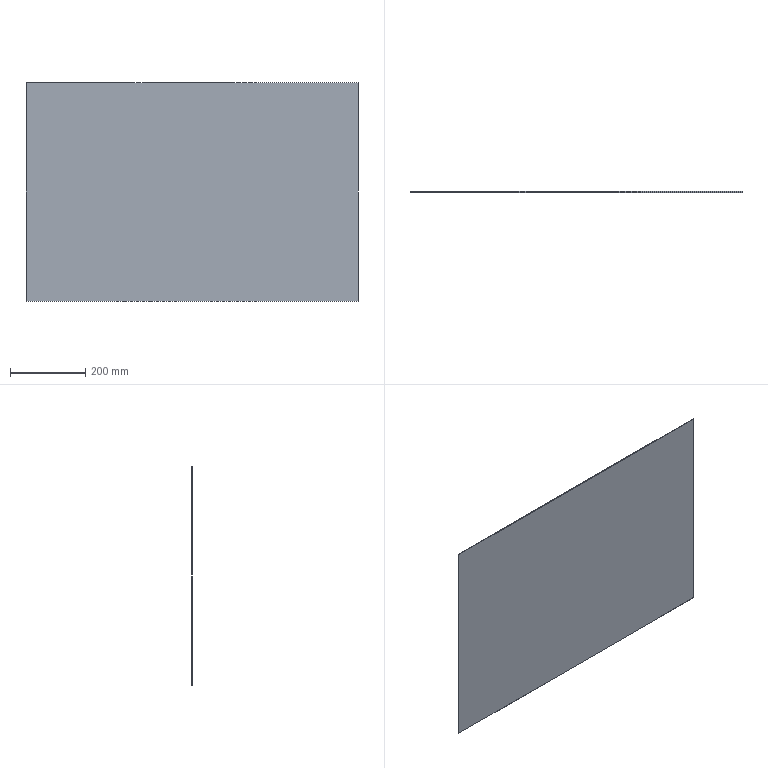Part | STEP file | 880X580 sealing plate | 1 solid | 6 faces | box 880 x 2 x 580 mm | volume 1020800 mm3 | plane 6
STEP:
#1=CARTESIAN_POINT('',(0.,0.,0.));
#2=DIRECTION('',(0.,0.,1.));
#3=DIRECTION('',(1.,0.,0.));
#4=AXIS2_PLACEMENT_3D('',#1,#2,#3);
#5=CARTESIAN_POINT('',(0.,0.,0.));
#6=VERTEX_POINT('',#5);
#7=CARTESIAN_POINT('',(0.,0.,580.));
#8=VERTEX_POINT('',#7);
#9=CARTESIAN_POINT('',(0.,0.,0.));
#10=DIRECTION('',(0.,0.,1.));
#11=VECTOR('',#10,1.);
#12=LINE('',#9,#11);
#13=CARTESIAN_POINT('',(0.,2.,0.));
#14=DIRECTION('',(1.,0.,0.));
#15=DIRECTION('',(0.,0.,-1.));
#16=AXIS2_PLACEMENT_3D('',#13,#14,#15);
#17=PLANE('',#16);
#18=CARTESIAN_POINT('',(0.,-2.));
#19=DIRECTION('',(-1.,0.));
#20=VECTOR('',#19,1.);
#21=LINE('',#18,#20);
#22=(GEOMETRIC_REPRESENTATION_CONTEXT(2)PARAMETRIC_REPRESENTATION_CONTEXT()REPRESENTATION_CONTEXT('',''));
#23=DEFINITIONAL_REPRESENTATION('',(#21),#22);
#24=PCURVE('',#17,#23);
#25=CARTESIAN_POINT('',(0.,0.,0.));
#26=DIRECTION('',(0.,1.,0.));
#27=DIRECTION('',(0.,0.,1.));
#28=AXIS2_PLACEMENT_3D('',#25,#26,#27);
#29=PLANE('',#28);
#30=CARTESIAN_POINT('',(0.,0.));
#31=DIRECTION('',(1.,0.));
#32=VECTOR('',#31,1.);
#33=LINE('',#30,#32);
#34=(GEOMETRIC_REPRESENTATION_CONTEXT(2)PARAMETRIC_REPRESENTATION_CONTEXT()REPRESENTATION_CONTEXT('',''));
#35=DEFINITIONAL_REPRESENTATION('',(#33),#34);
#36=PCURVE('',#29,#35);
#37=SURFACE_CURVE('',#12,(#24,#36),.PCURVE_S1.);
#38=EDGE_CURVE('',#6,#8,#37,.T.);
#39=ORIENTED_EDGE('',*,*,#38,.T.);
#40=CARTESIAN_POINT('',(0.,2.,580.));
#41=VERTEX_POINT('',#40);
#42=CARTESIAN_POINT('',(0.,2.,580.));
#43=DIRECTION('',(0.,-1.,0.));
#44=VECTOR('',#43,1.);
#45=LINE('',#42,#44);
#46=CARTESIAN_POINT('',(-580.,0.));
#47=DIRECTION('',(0.,-1.));
#48=VECTOR('',#47,1.);
#49=LINE('',#46,#48);
#50=(GEOMETRIC_REPRESENTATION_CONTEXT(2)PARAMETRIC_REPRESENTATION_CONTEXT()REPRESENTATION_CONTEXT('',''));
#51=DEFINITIONAL_REPRESENTATION('',(#49),#50);
#52=PCURVE('',#17,#51);
#53=CARTESIAN_POINT('',(0.,2.,580.));
#54=DIRECTION('',(0.,0.,-1.));
#55=DIRECTION('',(-1.,0.,0.));
#56=AXIS2_PLACEMENT_3D('',#53,#54,#55);
#57=PLANE('',#56);
#58=CARTESIAN_POINT('',(0.,0.));
#59=DIRECTION('',(0.,-1.));
#60=VECTOR('',#59,1.);
#61=LINE('',#58,#60);
#62=(GEOMETRIC_REPRESENTATION_CONTEXT(2)PARAMETRIC_REPRESENTATION_CONTEXT()REPRESENTATION_CONTEXT('',''));
#63=DEFINITIONAL_REPRESENTATION('',(#61),#62);
#64=PCURVE('',#57,#63);
#65=SURFACE_CURVE('',#45,(#52,#64),.PCURVE_S1.);
#66=EDGE_CURVE('',#41,#8,#65,.T.);
#67=ORIENTED_EDGE('',*,*,#66,.F.);
#68=CARTESIAN_POINT('',(0.,2.,0.));
#69=VERTEX_POINT('',#68);
#70=CARTESIAN_POINT('',(0.,2.,0.));
#71=DIRECTION('',(0.,0.,1.));
#72=VECTOR('',#71,1.);
#73=LINE('',#70,#72);
#74=CARTESIAN_POINT('',(0.,0.));
#75=DIRECTION('',(-1.,0.));
#76=VECTOR('',#75,1.);
#77=LINE('',#74,#76);
#78=(GEOMETRIC_REPRESENTATION_CONTEXT(2)PARAMETRIC_REPRESENTATION_CONTEXT()REPRESENTATION_CONTEXT('',''));
#79=DEFINITIONAL_REPRESENTATION('',(#77),#78);
#80=PCURVE('',#17,#79);
#81=CARTESIAN_POINT('',(0.,2.,0.));
#82=DIRECTION('',(0.,1.,0.));
#83=DIRECTION('',(0.,0.,1.));
#84=AXIS2_PLACEMENT_3D('',#81,#82,#83);
#85=PLANE('',#84);
#86=CARTESIAN_POINT('',(0.,0.));
#87=DIRECTION('',(1.,0.));
#88=VECTOR('',#87,1.);
#89=LINE('',#86,#88);
#90=(GEOMETRIC_REPRESENTATION_CONTEXT(2)PARAMETRIC_REPRESENTATION_CONTEXT()REPRESENTATION_CONTEXT('',''));
#91=DEFINITIONAL_REPRESENTATION('',(#89),#90);
#92=PCURVE('',#85,#91);
#93=SURFACE_CURVE('',#73,(#80,#92),.PCURVE_S1.);
#94=EDGE_CURVE('',#69,#41,#93,.T.);
#95=ORIENTED_EDGE('',*,*,#94,.F.);
#96=CARTESIAN_POINT('',(0.,2.,0.));
#97=DIRECTION('',(0.,-1.,0.));
#98=VECTOR('',#97,1.);
#99=LINE('',#96,#98);
#100=CARTESIAN_POINT('',(0.,0.));
#101=DIRECTION('',(0.,-1.));
#102=VECTOR('',#101,1.);
#103=LINE('',#100,#102);
#104=(GEOMETRIC_REPRESENTATION_CONTEXT(2)PARAMETRIC_REPRESENTATION_CONTEXT()REPRESENTATION_CONTEXT('',''));
#105=DEFINITIONAL_REPRESENTATION('',(#103),#104);
#106=PCURVE('',#17,#105);
#107=CARTESIAN_POINT('',(0.,2.,0.));
#108=DIRECTION('',(0.,0.,1.));
#109=DIRECTION('',(1.,0.,0.));
#110=AXIS2_PLACEMENT_3D('',#107,#108,#109);
#111=PLANE('',#110);
#112=CARTESIAN_POINT('',(0.,0.));
#113=DIRECTION('',(0.,-1.));
#114=VECTOR('',#113,1.);
#115=LINE('',#112,#114);
#116=(GEOMETRIC_REPRESENTATION_CONTEXT(2)PARAMETRIC_REPRESENTATION_CONTEXT()REPRESENTATION_CONTEXT('',''));
#117=DEFINITIONAL_REPRESENTATION('',(#115),#116);
#118=PCURVE('',#111,#117);
#119=SURFACE_CURVE('',#99,(#106,#118),.PCURVE_S1.);
#120=EDGE_CURVE('',#69,#6,#119,.T.);
#121=ORIENTED_EDGE('',*,*,#120,.T.);
#122=EDGE_LOOP('',(#39,#67,#95,#121));
#123=FACE_BOUND('',#122,.T.);
#124=ADVANCED_FACE('',(#123),#17,.F.);
#125=CARTESIAN_POINT('',(880.,0.,580.));
#126=VERTEX_POINT('',#125);
#127=CARTESIAN_POINT('',(0.,0.,580.));
#128=DIRECTION('',(1.,0.,0.));
#129=VECTOR('',#128,1.);
#130=LINE('',#127,#129);
#131=CARTESIAN_POINT('',(0.,-2.));
#132=DIRECTION('',(-1.,0.));
#133=VECTOR('',#132,1.);
#134=LINE('',#131,#133);
#135=(GEOMETRIC_REPRESENTATION_CONTEXT(2)PARAMETRIC_REPRESENTATION_CONTEXT()REPRESENTATION_CONTEXT('',''));
#136=DEFINITIONAL_REPRESENTATION('',(#134),#135);
#137=PCURVE('',#57,#136);
#138=CARTESIAN_POINT('',(580.,0.));
#139=DIRECTION('',(0.,1.));
#140=VECTOR('',#139,1.);
#141=LINE('',#138,#140);
#142=(GEOMETRIC_REPRESENTATION_CONTEXT(2)PARAMETRIC_REPRESENTATION_CONTEXT()REPRESENTATION_CONTEXT('',''));
#143=DEFINITIONAL_REPRESENTATION('',(#141),#142);
#144=PCURVE('',#29,#143);
#145=SURFACE_CURVE('',#130,(#137,#144),.PCURVE_S1.);
#146=EDGE_CURVE('',#8,#126,#145,.T.);
#147=ORIENTED_EDGE('',*,*,#146,.T.);
#148=CARTESIAN_POINT('',(880.,2.,580.));
#149=VERTEX_POINT('',#148);
#150=CARTESIAN_POINT('',(880.,2.,580.));
#151=DIRECTION('',(0.,-1.,0.));
#152=VECTOR('',#151,1.);
#153=LINE('',#150,#152);
#154=CARTESIAN_POINT('',(-880.,0.));
#155=DIRECTION('',(0.,-1.));
#156=VECTOR('',#155,1.);
#157=LINE('',#154,#156);
#158=(GEOMETRIC_REPRESENTATION_CONTEXT(2)PARAMETRIC_REPRESENTATION_CONTEXT()REPRESENTATION_CONTEXT('',''));
#159=DEFINITIONAL_REPRESENTATION('',(#157),#158);
#160=PCURVE('',#57,#159);
#161=CARTESIAN_POINT('',(880.,2.,0.));
#162=DIRECTION('',(-1.,0.,0.));
#163=DIRECTION('',(0.,0.,1.));
#164=AXIS2_PLACEMENT_3D('',#161,#162,#163);
#165=PLANE('',#164);
#166=CARTESIAN_POINT('',(580.,0.));
#167=DIRECTION('',(0.,-1.));
#168=VECTOR('',#167,1.);
#169=LINE('',#166,#168);
#170=(GEOMETRIC_REPRESENTATION_CONTEXT(2)PARAMETRIC_REPRESENTATION_CONTEXT()REPRESENTATION_CONTEXT('',''));
#171=DEFINITIONAL_REPRESENTATION('',(#169),#170);
#172=PCURVE('',#165,#171);
#173=SURFACE_CURVE('',#153,(#160,#172),.PCURVE_S1.);
#174=EDGE_CURVE('',#149,#126,#173,.T.);
#175=ORIENTED_EDGE('',*,*,#174,.F.);
#176=CARTESIAN_POINT('',(0.,2.,580.));
#177=DIRECTION('',(1.,0.,0.));
#178=VECTOR('',#177,1.);
#179=LINE('',#176,#178);
#180=CARTESIAN_POINT('',(0.,0.));
#181=DIRECTION('',(-1.,0.));
#182=VECTOR('',#181,1.);
#183=LINE('',#180,#182);
#184=(GEOMETRIC_REPRESENTATION_CONTEXT(2)PARAMETRIC_REPRESENTATION_CONTEXT()REPRESENTATION_CONTEXT('',''));
#185=DEFINITIONAL_REPRESENTATION('',(#183),#184);
#186=PCURVE('',#57,#185);
#187=CARTESIAN_POINT('',(580.,0.));
#188=DIRECTION('',(0.,1.));
#189=VECTOR('',#188,1.);
#190=LINE('',#187,#189);
#191=(GEOMETRIC_REPRESENTATION_CONTEXT(2)PARAMETRIC_REPRESENTATION_CONTEXT()REPRESENTATION_CONTEXT('',''));
#192=DEFINITIONAL_REPRESENTATION('',(#190),#191);
#193=PCURVE('',#85,#192);
#194=SURFACE_CURVE('',#179,(#186,#193),.PCURVE_S1.);
#195=EDGE_CURVE('',#41,#149,#194,.T.);
#196=ORIENTED_EDGE('',*,*,#195,.F.);
#197=ORIENTED_EDGE('',*,*,#66,.T.);
#198=EDGE_LOOP('',(#147,#175,#196,#197));
#199=FACE_BOUND('',#198,.T.);
#200=ADVANCED_FACE('',(#199),#57,.F.);
#201=CARTESIAN_POINT('',(880.,0.,0.));
#202=VERTEX_POINT('',#201);
#203=CARTESIAN_POINT('',(880.,0.,0.));
#204=DIRECTION('',(0.,0.,-1.));
#205=VECTOR('',#204,1.);
#206=LINE('',#203,#205);
#207=CARTESIAN_POINT('',(0.,-2.));
#208=DIRECTION('',(-1.,0.));
#209=VECTOR('',#208,1.);
#210=LINE('',#207,#209);
#211=(GEOMETRIC_REPRESENTATION_CONTEXT(2)PARAMETRIC_REPRESENTATION_CONTEXT()REPRESENTATION_CONTEXT('',''));
#212=DEFINITIONAL_REPRESENTATION('',(#210),#211);
#213=PCURVE('',#165,#212);
#214=CARTESIAN_POINT('',(0.,880.));
#215=DIRECTION('',(-1.,0.));
#216=VECTOR('',#215,1.);
#217=LINE('',#214,#216);
#218=(GEOMETRIC_REPRESENTATION_CONTEXT(2)PARAMETRIC_REPRESENTATION_CONTEXT()REPRESENTATION_CONTEXT('',''));
#219=DEFINITIONAL_REPRESENTATION('',(#217),#218);
#220=PCURVE('',#29,#219);
#221=SURFACE_CURVE('',#206,(#213,#220),.PCURVE_S1.);
#222=EDGE_CURVE('',#126,#202,#221,.T.);
#223=ORIENTED_EDGE('',*,*,#222,.T.);
#224=CARTESIAN_POINT('',(880.,2.,0.));
#225=VERTEX_POINT('',#224);
#226=CARTESIAN_POINT('',(880.,2.,0.));
#227=DIRECTION('',(0.,-1.,0.));
#228=VECTOR('',#227,1.);
#229=LINE('',#226,#228);
#230=CARTESIAN_POINT('',(0.,0.));
#231=DIRECTION('',(0.,-1.));
#232=VECTOR('',#231,1.);
#233=LINE('',#230,#232);
#234=(GEOMETRIC_REPRESENTATION_CONTEXT(2)PARAMETRIC_REPRESENTATION_CONTEXT()REPRESENTATION_CONTEXT('',''));
#235=DEFINITIONAL_REPRESENTATION('',(#233),#234);
#236=PCURVE('',#165,#235);
#237=CARTESIAN_POINT('',(880.,0.));
#238=DIRECTION('',(0.,-1.));
#239=VECTOR('',#238,1.);
#240=LINE('',#237,#239);
#241=(GEOMETRIC_REPRESENTATION_CONTEXT(2)PARAMETRIC_REPRESENTATION_CONTEXT()REPRESENTATION_CONTEXT('',''));
#242=DEFINITIONAL_REPRESENTATION('',(#240),#241);
#243=PCURVE('',#111,#242);
#244=SURFACE_CURVE('',#229,(#236,#243),.PCURVE_S1.);
#245=EDGE_CURVE('',#225,#202,#244,.T.);
#246=ORIENTED_EDGE('',*,*,#245,.F.);
#247=CARTESIAN_POINT('',(880.,2.,0.));
#248=DIRECTION('',(0.,0.,-1.));
#249=VECTOR('',#248,1.);
#250=LINE('',#247,#249);
#251=CARTESIAN_POINT('',(0.,0.));
#252=DIRECTION('',(-1.,0.));
#253=VECTOR('',#252,1.);
#254=LINE('',#251,#253);
#255=(GEOMETRIC_REPRESENTATION_CONTEXT(2)PARAMETRIC_REPRESENTATION_CONTEXT()REPRESENTATION_CONTEXT('',''));
#256=DEFINITIONAL_REPRESENTATION('',(#254),#255);
#257=PCURVE('',#165,#256);
#258=CARTESIAN_POINT('',(0.,880.));
#259=DIRECTION('',(-1.,0.));
#260=VECTOR('',#259,1.);
#261=LINE('',#258,#260);
#262=(GEOMETRIC_REPRESENTATION_CONTEXT(2)PARAMETRIC_REPRESENTATION_CONTEXT()REPRESENTATION_CONTEXT('',''));
#263=DEFINITIONAL_REPRESENTATION('',(#261),#262);
#264=PCURVE('',#85,#263);
#265=SURFACE_CURVE('',#250,(#257,#264),.PCURVE_S1.);
#266=EDGE_CURVE('',#149,#225,#265,.T.);
#267=ORIENTED_EDGE('',*,*,#266,.F.);
#268=ORIENTED_EDGE('',*,*,#174,.T.);
#269=EDGE_LOOP('',(#223,#246,#267,#268));
#270=FACE_BOUND('',#269,.T.);
#271=ADVANCED_FACE('',(#270),#165,.F.);
#272=CARTESIAN_POINT('',(0.,0.,0.));
#273=DIRECTION('',(-1.,0.,0.));
#274=VECTOR('',#273,1.);
#275=LINE('',#272,#274);
#276=CARTESIAN_POINT('',(0.,-2.));
#277=DIRECTION('',(-1.,0.));
#278=VECTOR('',#277,1.);
#279=LINE('',#276,#278);
#280=(GEOMETRIC_REPRESENTATION_CONTEXT(2)PARAMETRIC_REPRESENTATION_CONTEXT()REPRESENTATION_CONTEXT('',''));
#281=DEFINITIONAL_REPRESENTATION('',(#279),#280);
#282=PCURVE('',#111,#281);
#283=CARTESIAN_POINT('',(0.,0.));
#284=DIRECTION('',(0.,-1.));
#285=VECTOR('',#284,1.);
#286=LINE('',#283,#285);
#287=(GEOMETRIC_REPRESENTATION_CONTEXT(2)PARAMETRIC_REPRESENTATION_CONTEXT()REPRESENTATION_CONTEXT('',''));
#288=DEFINITIONAL_REPRESENTATION('',(#286),#287);
#289=PCURVE('',#29,#288);
#290=SURFACE_CURVE('',#275,(#282,#289),.PCURVE_S1.);
#291=EDGE_CURVE('',#202,#6,#290,.T.);
#292=ORIENTED_EDGE('',*,*,#291,.T.);
#293=ORIENTED_EDGE('',*,*,#120,.F.);
#294=CARTESIAN_POINT('',(0.,2.,0.));
#295=DIRECTION('',(-1.,0.,0.));
#296=VECTOR('',#295,1.);
#297=LINE('',#294,#296);
#298=CARTESIAN_POINT('',(0.,0.));
#299=DIRECTION('',(-1.,0.));
#300=VECTOR('',#299,1.);
#301=LINE('',#298,#300);
#302=(GEOMETRIC_REPRESENTATION_CONTEXT(2)PARAMETRIC_REPRESENTATION_CONTEXT()REPRESENTATION_CONTEXT('',''));
#303=DEFINITIONAL_REPRESENTATION('',(#301),#302);
#304=PCURVE('',#111,#303);
#305=CARTESIAN_POINT('',(0.,0.));
#306=DIRECTION('',(0.,-1.));
#307=VECTOR('',#306,1.);
#308=LINE('',#305,#307);
#309=(GEOMETRIC_REPRESENTATION_CONTEXT(2)PARAMETRIC_REPRESENTATION_CONTEXT()REPRESENTATION_CONTEXT('',''));
#310=DEFINITIONAL_REPRESENTATION('',(#308),#309);
#311=PCURVE('',#85,#310);
#312=SURFACE_CURVE('',#297,(#304,#311),.PCURVE_S1.);
#313=EDGE_CURVE('',#225,#69,#312,.T.);
#314=ORIENTED_EDGE('',*,*,#313,.F.);
#315=ORIENTED_EDGE('',*,*,#245,.T.);
#316=EDGE_LOOP('',(#292,#293,#314,#315));
#317=FACE_BOUND('',#316,.T.);
#318=ADVANCED_FACE('',(#317),#111,.F.);
#319=ORIENTED_EDGE('',*,*,#94,.T.);
#320=ORIENTED_EDGE('',*,*,#195,.T.);
#321=ORIENTED_EDGE('',*,*,#266,.T.);
#322=ORIENTED_EDGE('',*,*,#313,.T.);
#323=EDGE_LOOP('',(#319,#320,#321,#322));
#324=FACE_BOUND('',#323,.T.);
#325=ADVANCED_FACE('',(#324),#85,.T.);
#326=ORIENTED_EDGE('',*,*,#38,.F.);
#327=ORIENTED_EDGE('',*,*,#291,.F.);
#328=ORIENTED_EDGE('',*,*,#222,.F.);
#329=ORIENTED_EDGE('',*,*,#146,.F.);
#330=EDGE_LOOP('',(#326,#327,#328,#329));
#331=FACE_BOUND('',#330,.T.);
#332=ADVANCED_FACE('',(#331),#29,.F.);
#333=CLOSED_SHELL('',(#124,#200,#271,#318,#325,#332));
#334=MANIFOLD_SOLID_BREP('',#333);
#335=(LENGTH_UNIT()NAMED_UNIT(*)SI_UNIT(.MILLI.,.METRE.));
#336=UNCERTAINTY_MEASURE_WITH_UNIT(LENGTH_MEASURE(0.0000001),#335,'','');
#337=(NAMED_UNIT(*)PLANE_ANGLE_UNIT()SI_UNIT($,.RADIAN.));
#338=(NAMED_UNIT(*)SI_UNIT($,.STERADIAN.)SOLID_ANGLE_UNIT());
#339=(GEOMETRIC_REPRESENTATION_CONTEXT(3)GLOBAL_UNCERTAINTY_ASSIGNED_CONTEXT((#336))GLOBAL_UNIT_ASSIGNED_CONTEXT((#335,#337,#338))REPRESENTATION_CONTEXT('',''));
#340=ADVANCED_BREP_SHAPE_REPRESENTATION('',(#4,#334),#339);